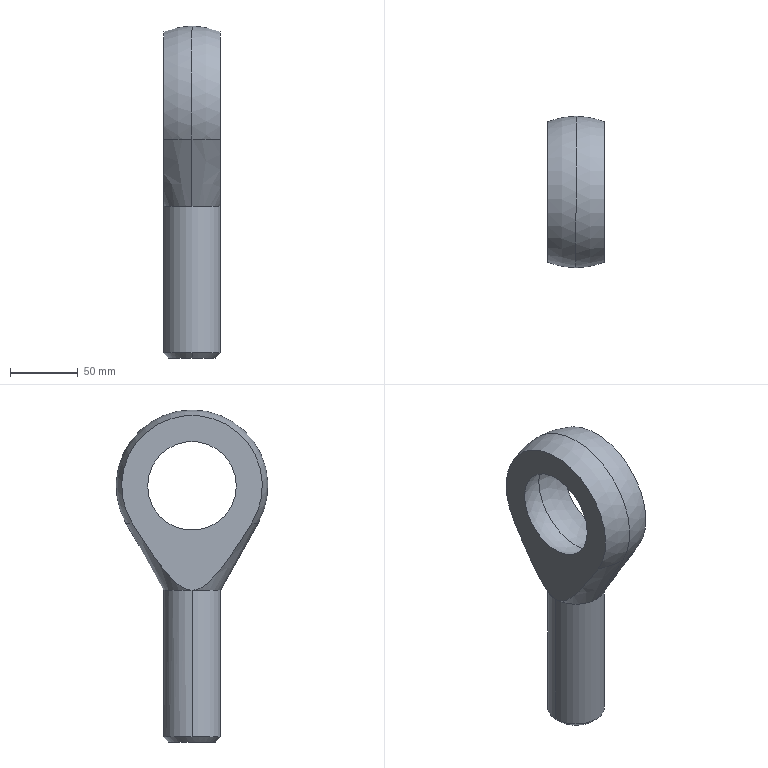Part | STEP file | Traction rod end | 1 solid | 14 faces | box 42 x 112 x 245 mm | volume 426798 mm3 | cone 5 | sphere 4 | plane 3 | cylinder 2 | commonest cylinder face diameters 42 x2
STEP:
#1=CARTESIAN_POINT('',(0.,-21.,224.245));
#2=VERTEX_POINT('',#1);
#3=CARTESIAN_POINT('',(-21.,0.,224.245));
#4=VERTEX_POINT('',#3);
#5=CARTESIAN_POINT('',(0.,0.,224.245));
#6=DIRECTION('',(0.,0.,-1.));
#7=DIRECTION('',(1.,0.,0.));
#8=AXIS2_PLACEMENT_3D('',#5,#6,#7);
#9=CIRCLE('',#8,21.);
#10=EDGE_CURVE('',#2,#4,#9,.T.);
#11=ORIENTED_EDGE('',*,*,#10,.T.);
#12=CARTESIAN_POINT('',(-21.,0.,116.002));
#13=VERTEX_POINT('',#12);
#14=CARTESIAN_POINT('',(-21.,0.,112.245));
#15=DIRECTION('',(0.,0.,-1.));
#16=VECTOR('',#15,1000.);
#17=LINE('',#14,#16);
#18=EDGE_CURVE('',#4,#13,#17,.T.);
#19=ORIENTED_EDGE('',*,*,#18,.T.);
#20=CARTESIAN_POINT('',(0.,-21.,116.002));
#21=VERTEX_POINT('',#20);
#22=CARTESIAN_POINT('',(0.,0.,116.002));
#23=DIRECTION('',(0.,0.,1.));
#24=DIRECTION('',(1.,0.,0.));
#25=AXIS2_PLACEMENT_3D('',#22,#23,#24);
#26=CIRCLE('',#25,21.);
#27=EDGE_CURVE('',#13,#21,#26,.T.);
#28=ORIENTED_EDGE('',*,*,#27,.T.);
#29=CARTESIAN_POINT('',(21.,0.,116.002));
#30=VERTEX_POINT('',#29);
#31=CARTESIAN_POINT('',(0.,0.,116.002));
#32=DIRECTION('',(0.,0.,1.));
#33=DIRECTION('',(1.,0.,0.));
#34=AXIS2_PLACEMENT_3D('',#31,#32,#33);
#35=CIRCLE('',#34,21.);
#36=EDGE_CURVE('',#21,#30,#35,.T.);
#37=ORIENTED_EDGE('',*,*,#36,.T.);
#38=CARTESIAN_POINT('',(21.,0.,224.245));
#39=VERTEX_POINT('',#38);
#40=CARTESIAN_POINT('',(21.,0.,112.245));
#41=DIRECTION('',(0.,0.,-1.));
#42=VECTOR('',#41,1000.);
#43=LINE('',#40,#42);
#44=EDGE_CURVE('',#39,#30,#43,.T.);
#45=ORIENTED_EDGE('',*,*,#44,.F.);
#46=CARTESIAN_POINT('',(0.,0.,224.245));
#47=DIRECTION('',(0.,0.,-1.));
#48=DIRECTION('',(1.,0.,0.));
#49=AXIS2_PLACEMENT_3D('',#46,#47,#48);
#50=CIRCLE('',#49,21.);
#51=EDGE_CURVE('',#39,#2,#50,.T.);
#52=ORIENTED_EDGE('',*,*,#51,.T.);
#53=EDGE_LOOP('',(#11,#19,#28,#37,#45,#52));
#54=FACE_OUTER_BOUND('',#53,.T.);
#55=CARTESIAN_POINT('',(0.,0.,112.245));
#56=DIRECTION('',(0.,0.,-1.));
#57=DIRECTION('',(1.,0.,0.));
#58=AXIS2_PLACEMENT_3D('',#55,#56,#57);
#59=CYLINDRICAL_SURFACE('',#58,21.);
#60=ADVANCED_FACE('',(#54),#59,.T.);
#61=CARTESIAN_POINT('',(0.,-17.243,112.245));
#62=VERTEX_POINT('',#61);
#63=CARTESIAN_POINT('',(0.,17.243,112.245));
#64=VERTEX_POINT('',#63);
#65=CARTESIAN_POINT('',(0.,0.,112.245));
#66=DIRECTION('',(0.,0.,1.));
#67=DIRECTION('',(0.,-1.,0.));
#68=AXIS2_PLACEMENT_3D('',#65,#66,#67);
#69=CIRCLE('',#68,17.243);
#70=EDGE_CURVE('',#62,#64,#69,.T.);
#71=ORIENTED_EDGE('',*,*,#70,.T.);
#72=CARTESIAN_POINT('',(0.,21.,116.002));
#73=VERTEX_POINT('',#72);
#74=CARTESIAN_POINT('',(0.,21.,116.002));
#75=DIRECTION('',(0.,0.7071,0.7071));
#76=VECTOR('',#75,1000.);
#77=LINE('',#74,#76);
#78=EDGE_CURVE('',#64,#73,#77,.T.);
#79=ORIENTED_EDGE('',*,*,#78,.T.);
#80=CARTESIAN_POINT('',(0.,0.,116.002));
#81=DIRECTION('',(0.,0.,1.));
#82=DIRECTION('',(1.,0.,0.));
#83=AXIS2_PLACEMENT_3D('',#80,#81,#82);
#84=CIRCLE('',#83,21.);
#85=EDGE_CURVE('',#30,#73,#84,.T.);
#86=ORIENTED_EDGE('',*,*,#85,.F.);
#87=ORIENTED_EDGE('',*,*,#36,.F.);
#88=CARTESIAN_POINT('',(0.,-21.,116.002));
#89=DIRECTION('',(0.,-0.7071,0.7071));
#90=VECTOR('',#89,1000.);
#91=LINE('',#88,#90);
#92=EDGE_CURVE('',#62,#21,#91,.T.);
#93=ORIENTED_EDGE('',*,*,#92,.F.);
#94=EDGE_LOOP('',(#71,#79,#86,#87,#93));
#95=FACE_OUTER_BOUND('',#94,.T.);
#96=CARTESIAN_POINT('',(0.,0.,116.002));
#97=DIRECTION('',(0.,0.,1.));
#98=DIRECTION('',(0.,-1.,0.));
#99=AXIS2_PLACEMENT_3D('',#96,#97,#98);
#100=CONICAL_SURFACE('',#99,21.,0.7854);
#101=ADVANCED_FACE('',(#95),#100,.T.);
#102=ORIENTED_EDGE('',*,*,#10,.F.);
#103=CARTESIAN_POINT('',(0.,-48.834,273.836));
#104=VERTEX_POINT('',#103);
#105=CARTESIAN_POINT('',(0.,-48.834,273.836));
#106=DIRECTION('',(0.,-0.4894,0.872));
#107=VECTOR('',#106,1000.);
#108=LINE('',#105,#107);
#109=EDGE_CURVE('',#2,#104,#108,.T.);
#110=ORIENTED_EDGE('',*,*,#109,.T.);
#111=CARTESIAN_POINT('',(-21.,-44.088,273.836));
#112=VERTEX_POINT('',#111);
#113=CARTESIAN_POINT('',(0.,0.,273.836));
#114=DIRECTION('',(0.,0.,-1.));
#115=DIRECTION('',(1.,0.,0.));
#116=AXIS2_PLACEMENT_3D('',#113,#114,#115);
#117=CIRCLE('',#116,48.834);
#118=EDGE_CURVE('',#104,#112,#117,.T.);
#119=ORIENTED_EDGE('',*,*,#118,.T.);
#120=CARTESIAN_POINT('',(-21.,-44.088,273.836));
#121=CARTESIAN_POINT('',(-21.,-41.092,269.018));
#122=CARTESIAN_POINT('',(-21.,-38.059,264.224));
#123=CARTESIAN_POINT('',(-21.,-33.398,257.105));
#124=CARTESIAN_POINT('',(-21.,-31.825,254.744));
#125=CARTESIAN_POINT('',(-21.,-28.623,250.059));
#126=CARTESIAN_POINT('',(-21.,-26.995,247.737));
#127=CARTESIAN_POINT('',(-21.,-23.654,243.154));
#128=CARTESIAN_POINT('',(-21.,-21.94,240.891));
#129=CARTESIAN_POINT('',(-21.,-19.26,237.586));
#130=CARTESIAN_POINT('',(-21.,-18.35,236.5));
#131=CARTESIAN_POINT('',(-21.,-16.482,234.375));
#132=CARTESIAN_POINT('',(-21.,-15.524,233.335));
#133=CARTESIAN_POINT('',(-21.,-13.538,231.323));
#134=CARTESIAN_POINT('',(-21.,-12.511,230.349));
#135=CARTESIAN_POINT('',(-21.,-10.889,228.967));
#136=CARTESIAN_POINT('',(-21.,-10.333,228.519));
#137=CARTESIAN_POINT('',(-21.,-9.193,227.663));
#138=CARTESIAN_POINT('',(-21.,-8.61,227.255));
#139=CARTESIAN_POINT('',(-21.,-7.411,226.494));
#140=CARTESIAN_POINT('',(-21.,-6.796,226.14));
#141=CARTESIAN_POINT('',(-21.,-5.522,225.502));
#142=CARTESIAN_POINT('',(-21.,-4.861,225.217));
#143=CARTESIAN_POINT('',(-21.,-3.519,224.749));
#144=CARTESIAN_POINT('',(-21.,-2.836,224.564));
#145=CARTESIAN_POINT('',(-21.,-1.438,224.312));
#146=CARTESIAN_POINT('',(-21.,-0.719,224.245));
#147=CARTESIAN_POINT('',(-21.,0.,224.245));
#148=B_SPLINE_CURVE_WITH_KNOTS('',3,(#120,#121,#122,#123,#124,#125,#126,#127,#128,#129,#130,#131,#132,#133,#134,#135,#136,#137,#138,#139,#140,#141,#142,#143,#144,#145,#146,#147),.UNSPECIFIED.,.F.,.F.,(4,2,2,2,2,2,2,2,2,2,2,2,2,4),(0.,0.01702,0.02553,0.03404,0.04255,0.0468,0.05105,0.05531,0.05744,0.05956,0.06169,0.06382,0.06595,0.06807),.UNSPECIFIED.);
#149=EDGE_CURVE('',#112,#4,#148,.T.);
#150=ORIENTED_EDGE('',*,*,#149,.T.);
#151=EDGE_LOOP('',(#102,#110,#119,#150));
#152=FACE_OUTER_BOUND('',#151,.T.);
#153=CARTESIAN_POINT('',(0.,0.,273.836));
#154=DIRECTION('',(0.,0.,1.));
#155=DIRECTION('',(0.,-1.,0.));
#156=AXIS2_PLACEMENT_3D('',#153,#154,#155);
#157=CONICAL_SURFACE('',#156,48.834,0.5115);
#158=ADVANCED_FACE('',(#152),#157,.T.);
#159=CARTESIAN_POINT('',(0.,48.834,273.836));
#160=VERTEX_POINT('',#159);
#161=CARTESIAN_POINT('',(21.,44.088,273.836));
#162=VERTEX_POINT('',#161);
#163=CARTESIAN_POINT('',(0.,0.,273.836));
#164=DIRECTION('',(0.,0.,-1.));
#165=DIRECTION('',(0.,-1.,0.));
#166=AXIS2_PLACEMENT_3D('',#163,#164,#165);
#167=CIRCLE('',#166,48.834);
#168=EDGE_CURVE('',#160,#162,#167,.T.);
#169=ORIENTED_EDGE('',*,*,#168,.F.);
#170=CARTESIAN_POINT('',(0.,0.,357.245));
#171=VERTEX_POINT('',#170);
#172=CARTESIAN_POINT('',(0.,0.,301.245));
#173=DIRECTION('',(1.,0.,0.));
#174=DIRECTION('',(0.,1.,0.));
#175=AXIS2_PLACEMENT_3D('',#172,#173,#174);
#176=CIRCLE('',#175,56.);
#177=EDGE_CURVE('',#160,#171,#176,.T.);
#178=ORIENTED_EDGE('',*,*,#177,.T.);
#179=CARTESIAN_POINT('',(0.,0.,301.245));
#180=DIRECTION('',(-1.,0.,0.));
#181=DIRECTION('',(0.,-1.,0.));
#182=AXIS2_PLACEMENT_3D('',#179,#180,#181);
#183=CIRCLE('',#182,56.);
#184=EDGE_CURVE('',#104,#171,#183,.T.);
#185=ORIENTED_EDGE('',*,*,#184,.F.);
#186=CARTESIAN_POINT('',(21.,-44.088,273.836));
#187=VERTEX_POINT('',#186);
#188=CARTESIAN_POINT('',(0.,0.,273.836));
#189=DIRECTION('',(0.,0.,-1.));
#190=DIRECTION('',(1.,0.,0.));
#191=AXIS2_PLACEMENT_3D('',#188,#189,#190);
#192=CIRCLE('',#191,48.834);
#193=EDGE_CURVE('',#187,#104,#192,.T.);
#194=ORIENTED_EDGE('',*,*,#193,.F.);
#195=CARTESIAN_POINT('',(21.,0.,301.245));
#196=DIRECTION('',(-1.,0.,0.));
#197=DIRECTION('',(0.,-1.,0.));
#198=AXIS2_PLACEMENT_3D('',#195,#196,#197);
#199=CIRCLE('',#198,51.913);
#200=EDGE_CURVE('',#187,#162,#199,.T.);
#201=ORIENTED_EDGE('',*,*,#200,.T.);
#202=EDGE_LOOP('',(#169,#178,#185,#194,#201));
#203=FACE_OUTER_BOUND('',#202,.T.);
#204=CARTESIAN_POINT('',(0.,0.,301.245));
#205=DIRECTION('',(1.,0.,0.));
#206=DIRECTION('',(0.,-1.,0.));
#207=AXIS2_PLACEMENT_3D('',#204,#205,#206);
#208=SPHERICAL_SURFACE('',#207,56.);
#209=ADVANCED_FACE('',(#203),#208,.T.);
#210=CARTESIAN_POINT('',(21.,-32.748,301.245));
#211=VERTEX_POINT('',#210);
#212=CARTESIAN_POINT('',(21.,32.748,301.245));
#213=VERTEX_POINT('',#212);
#214=CARTESIAN_POINT('',(21.,0.,301.245));
#215=DIRECTION('',(-1.,0.,0.));
#216=DIRECTION('',(0.,-1.,0.));
#217=AXIS2_PLACEMENT_3D('',#214,#215,#216);
#218=CIRCLE('',#217,32.748);
#219=EDGE_CURVE('',#211,#213,#218,.T.);
#220=ORIENTED_EDGE('',*,*,#219,.F.);
#221=CARTESIAN_POINT('',(21.,0.,301.245));
#222=DIRECTION('',(-1.,0.,0.));
#223=DIRECTION('',(0.,-1.,0.));
#224=AXIS2_PLACEMENT_3D('',#221,#222,#223);
#225=CIRCLE('',#224,32.748);
#226=EDGE_CURVE('',#213,#211,#225,.T.);
#227=ORIENTED_EDGE('',*,*,#226,.F.);
#228=EDGE_LOOP('',(#220,#227));
#229=FACE_BOUND('',#228,.T.);
#230=CARTESIAN_POINT('',(0.,0.,262.343));
#231=VERTEX_POINT('',#230);
#232=CARTESIAN_POINT('',(0.,0.,340.148));
#233=VERTEX_POINT('',#232);
#234=CARTESIAN_POINT('',(0.,0.,301.245));
#235=DIRECTION('',(1.,0.,0.));
#236=DIRECTION('',(0.,1.,0.));
#237=AXIS2_PLACEMENT_3D('',#234,#235,#236);
#238=CIRCLE('',#237,38.902);
#239=EDGE_CURVE('',#231,#233,#238,.T.);
#240=ORIENTED_EDGE('',*,*,#239,.F.);
#241=CARTESIAN_POINT('',(0.,0.,301.245));
#242=DIRECTION('',(-1.,0.,0.));
#243=DIRECTION('',(0.,-1.,0.));
#244=AXIS2_PLACEMENT_3D('',#241,#242,#243);
#245=CIRCLE('',#244,38.902);
#246=EDGE_CURVE('',#231,#233,#245,.T.);
#247=ORIENTED_EDGE('',*,*,#246,.T.);
#248=EDGE_LOOP('',(#240,#247));
#249=FACE_OUTER_BOUND('',#248,.T.);
#250=CARTESIAN_POINT('',(0.,0.,301.245));
#251=DIRECTION('',(-1.,0.,0.));
#252=DIRECTION('',(0.,1.,0.));
#253=AXIS2_PLACEMENT_3D('',#250,#251,#252);
#254=SPHERICAL_SURFACE('',#253,38.902);
#255=ADVANCED_FACE('',(#229,#249),#254,.F.);
#256=ORIENTED_EDGE('',*,*,#18,.F.);
#257=CARTESIAN_POINT('',(0.,0.,224.245));
#258=DIRECTION('',(0.,0.,-1.));
#259=DIRECTION('',(1.,0.,0.));
#260=AXIS2_PLACEMENT_3D('',#257,#258,#259);
#261=CIRCLE('',#260,21.);
#262=EDGE_CURVE('',#4,#39,#261,.T.);
#263=ORIENTED_EDGE('',*,*,#262,.T.);
#264=ORIENTED_EDGE('',*,*,#44,.T.);
#265=ORIENTED_EDGE('',*,*,#85,.T.);
#266=CARTESIAN_POINT('',(0.,0.,116.002));
#267=DIRECTION('',(0.,0.,1.));
#268=DIRECTION('',(1.,0.,0.));
#269=AXIS2_PLACEMENT_3D('',#266,#267,#268);
#270=CIRCLE('',#269,21.);
#271=EDGE_CURVE('',#73,#13,#270,.T.);
#272=ORIENTED_EDGE('',*,*,#271,.T.);
#273=EDGE_LOOP('',(#256,#263,#264,#265,#272));
#274=FACE_OUTER_BOUND('',#273,.T.);
#275=CARTESIAN_POINT('',(0.,0.,112.245));
#276=DIRECTION('',(0.,0.,-1.));
#277=DIRECTION('',(1.,0.,0.));
#278=AXIS2_PLACEMENT_3D('',#275,#276,#277);
#279=CYLINDRICAL_SURFACE('',#278,21.);
#280=ADVANCED_FACE('',(#274),#279,.T.);
#281=ORIENTED_EDGE('',*,*,#78,.F.);
#282=CARTESIAN_POINT('',(0.,0.,112.245));
#283=DIRECTION('',(0.,0.,1.));
#284=DIRECTION('',(0.,-1.,0.));
#285=AXIS2_PLACEMENT_3D('',#282,#283,#284);
#286=CIRCLE('',#285,17.243);
#287=EDGE_CURVE('',#64,#62,#286,.T.);
#288=ORIENTED_EDGE('',*,*,#287,.T.);
#289=ORIENTED_EDGE('',*,*,#92,.T.);
#290=ORIENTED_EDGE('',*,*,#27,.F.);
#291=ORIENTED_EDGE('',*,*,#271,.F.);
#292=EDGE_LOOP('',(#281,#288,#289,#290,#291));
#293=FACE_OUTER_BOUND('',#292,.T.);
#294=CARTESIAN_POINT('',(0.,0.,116.002));
#295=DIRECTION('',(0.,0.,1.));
#296=DIRECTION('',(0.,-1.,0.));
#297=AXIS2_PLACEMENT_3D('',#294,#295,#296);
#298=CONICAL_SURFACE('',#297,21.,0.7854);
#299=ADVANCED_FACE('',(#293),#298,.T.);
#300=ORIENTED_EDGE('',*,*,#109,.F.);
#301=ORIENTED_EDGE('',*,*,#51,.F.);
#302=CARTESIAN_POINT('',(21.,0.,224.245));
#303=CARTESIAN_POINT('',(21.,-1.452,224.245));
#304=CARTESIAN_POINT('',(21.,-2.851,224.514));
#305=CARTESIAN_POINT('',(21.,-4.549,225.108));
#306=CARTESIAN_POINT('',(21.,-4.887,225.241));
#307=CARTESIAN_POINT('',(21.,-5.549,225.525));
#308=CARTESIAN_POINT('',(21.,-5.873,225.677));
#309=CARTESIAN_POINT('',(21.,-6.831,226.16));
#310=CARTESIAN_POINT('',(21.,-7.449,226.517));
#311=CARTESIAN_POINT('',(21.,-8.652,227.284));
#312=CARTESIAN_POINT('',(21.,-9.237,227.694));
#313=CARTESIAN_POINT('',(21.,-10.382,228.557));
#314=CARTESIAN_POINT('',(21.,-10.942,229.011));
#315=CARTESIAN_POINT('',(21.,-12.573,230.405));
#316=CARTESIAN_POINT('',(21.,-13.601,231.384));
#317=CARTESIAN_POINT('',(21.,-15.586,233.402));
#318=CARTESIAN_POINT('',(21.,-16.542,234.442));
#319=CARTESIAN_POINT('',(21.,-18.404,236.564));
#320=CARTESIAN_POINT('',(21.,-19.31,237.646));
#321=CARTESIAN_POINT('',(21.,-21.974,240.936));
#322=CARTESIAN_POINT('',(21.,-23.681,243.189));
#323=CARTESIAN_POINT('',(21.,-27.013,247.762));
#324=CARTESIAN_POINT('',(21.,-28.64,250.084));
#325=CARTESIAN_POINT('',(21.,-31.838,254.764));
#326=CARTESIAN_POINT('',(21.,-33.409,257.122));
#327=CARTESIAN_POINT('',(21.,-38.065,264.234));
#328=CARTESIAN_POINT('',(21.,-41.095,269.023));
#329=CARTESIAN_POINT('',(21.,-44.088,273.836));
#330=B_SPLINE_CURVE_WITH_KNOTS('',3,(#302,#303,#304,#305,#306,#307,#308,#309,#310,#311,#312,#313,#314,#315,#316,#317,#318,#319,#320,#321,#322,#323,#324,#325,#326,#327,#328,#329),.UNSPECIFIED.,.F.,.F.,(4,2,2,2,2,2,2,2,2,2,2,2,2,4),(0.,0.004274,0.005342,0.006411,0.008548,0.01068,0.01282,0.0171,0.02137,0.02564,0.03419,0.04274,0.05129,0.06838),.UNSPECIFIED.);
#331=EDGE_CURVE('',#39,#187,#330,.T.);
#332=ORIENTED_EDGE('',*,*,#331,.T.);
#333=ORIENTED_EDGE('',*,*,#193,.T.);
#334=EDGE_LOOP('',(#300,#301,#332,#333));
#335=FACE_OUTER_BOUND('',#334,.T.);
#336=CARTESIAN_POINT('',(0.,0.,273.836));
#337=DIRECTION('',(0.,0.,1.));
#338=DIRECTION('',(0.,-1.,0.));
#339=AXIS2_PLACEMENT_3D('',#336,#337,#338);
#340=CONICAL_SURFACE('',#339,48.834,0.5115);
#341=ADVANCED_FACE('',(#335),#340,.T.);
#342=ORIENTED_EDGE('',*,*,#70,.F.);
#343=ORIENTED_EDGE('',*,*,#287,.F.);
#344=EDGE_LOOP('',(#342,#343));
#345=FACE_OUTER_BOUND('',#344,.T.);
#346=CARTESIAN_POINT('',(-17.243,0.,112.245));
#347=DIRECTION('',(0.,0.,1.));
#348=DIRECTION('',(-1.,0.,0.));
#349=AXIS2_PLACEMENT_3D('',#346,#347,#348);
#350=PLANE('',#349);
#351=ADVANCED_FACE('',(#345),#350,.F.);
#352=CARTESIAN_POINT('',(21.,44.088,273.836));
#353=CARTESIAN_POINT('',(21.,41.092,269.018));
#354=CARTESIAN_POINT('',(21.,38.059,264.224));
#355=CARTESIAN_POINT('',(21.,33.398,257.105));
#356=CARTESIAN_POINT('',(21.,31.825,254.744));
#357=CARTESIAN_POINT('',(21.,28.623,250.059));
#358=CARTESIAN_POINT('',(21.,26.995,247.737));
#359=CARTESIAN_POINT('',(21.,23.654,243.154));
#360=CARTESIAN_POINT('',(21.,21.94,240.891));
#361=CARTESIAN_POINT('',(21.,19.26,237.586));
#362=CARTESIAN_POINT('',(21.,18.35,236.5));
#363=CARTESIAN_POINT('',(21.,16.482,234.375));
#364=CARTESIAN_POINT('',(21.,15.524,233.335));
#365=CARTESIAN_POINT('',(21.,13.538,231.323));
#366=CARTESIAN_POINT('',(21.,12.511,230.349));
#367=CARTESIAN_POINT('',(21.,10.889,228.967));
#368=CARTESIAN_POINT('',(21.,10.333,228.519));
#369=CARTESIAN_POINT('',(21.,9.193,227.663));
#370=CARTESIAN_POINT('',(21.,8.61,227.255));
#371=CARTESIAN_POINT('',(21.,7.411,226.494));
#372=CARTESIAN_POINT('',(21.,6.796,226.14));
#373=CARTESIAN_POINT('',(21.,5.522,225.502));
#374=CARTESIAN_POINT('',(21.,4.861,225.217));
#375=CARTESIAN_POINT('',(21.,3.519,224.749));
#376=CARTESIAN_POINT('',(21.,2.836,224.564));
#377=CARTESIAN_POINT('',(21.,1.438,224.312));
#378=CARTESIAN_POINT('',(21.,0.719,224.245));
#379=CARTESIAN_POINT('',(21.,0.,224.245));
#380=B_SPLINE_CURVE_WITH_KNOTS('',3,(#352,#353,#354,#355,#356,#357,#358,#359,#360,#361,#362,#363,#364,#365,#366,#367,#368,#369,#370,#371,#372,#373,#374,#375,#376,#377,#378,#379),.UNSPECIFIED.,.F.,.F.,(4,2,2,2,2,2,2,2,2,2,2,2,2,4),(0.,0.01702,0.02553,0.03404,0.04255,0.0468,0.05105,0.05531,0.05744,0.05956,0.06169,0.06382,0.06595,0.06807),.UNSPECIFIED.);
#381=EDGE_CURVE('',#162,#39,#380,.T.);
#382=ORIENTED_EDGE('',*,*,#381,.T.);
#383=ORIENTED_EDGE('',*,*,#262,.F.);
#384=CARTESIAN_POINT('',(-21.,44.088,273.836));
#385=VERTEX_POINT('',#384);
#386=CARTESIAN_POINT('',(-21.,0.,224.245));
#387=CARTESIAN_POINT('',(-21.,1.452,224.245));
#388=CARTESIAN_POINT('',(-21.,2.851,224.514));
#389=CARTESIAN_POINT('',(-21.,4.549,225.108));
#390=CARTESIAN_POINT('',(-21.,4.887,225.241));
#391=CARTESIAN_POINT('',(-21.,5.549,225.525));
#392=CARTESIAN_POINT('',(-21.,5.873,225.677));
#393=CARTESIAN_POINT('',(-21.,6.831,226.16));
#394=CARTESIAN_POINT('',(-21.,7.449,226.517));
#395=CARTESIAN_POINT('',(-21.,8.652,227.284));
#396=CARTESIAN_POINT('',(-21.,9.237,227.694));
#397=CARTESIAN_POINT('',(-21.,10.382,228.557));
#398=CARTESIAN_POINT('',(-21.,10.942,229.011));
#399=CARTESIAN_POINT('',(-21.,12.573,230.405));
#400=CARTESIAN_POINT('',(-21.,13.601,231.384));
#401=CARTESIAN_POINT('',(-21.,15.586,233.402));
#402=CARTESIAN_POINT('',(-21.,16.542,234.442));
#403=CARTESIAN_POINT('',(-21.,18.404,236.564));
#404=CARTESIAN_POINT('',(-21.,19.31,237.646));
#405=CARTESIAN_POINT('',(-21.,21.974,240.936));
#406=CARTESIAN_POINT('',(-21.,23.681,243.189));
#407=CARTESIAN_POINT('',(-21.,27.013,247.762));
#408=CARTESIAN_POINT('',(-21.,28.64,250.084));
#409=CARTESIAN_POINT('',(-21.,31.838,254.764));
#410=CARTESIAN_POINT('',(-21.,33.409,257.122));
#411=CARTESIAN_POINT('',(-21.,38.065,264.234));
#412=CARTESIAN_POINT('',(-21.,41.095,269.023));
#413=CARTESIAN_POINT('',(-21.,44.088,273.836));
#414=B_SPLINE_CURVE_WITH_KNOTS('',3,(#386,#387,#388,#389,#390,#391,#392,#393,#394,#395,#396,#397,#398,#399,#400,#401,#402,#403,#404,#405,#406,#407,#408,#409,#410,#411,#412,#413),.UNSPECIFIED.,.F.,.F.,(4,2,2,2,2,2,2,2,2,2,2,2,2,4),(0.,0.004274,0.005342,0.006411,0.008548,0.01068,0.01282,0.0171,0.02137,0.02564,0.03419,0.04274,0.05129,0.06838),.UNSPECIFIED.);
#415=EDGE_CURVE('',#4,#385,#414,.T.);
#416=ORIENTED_EDGE('',*,*,#415,.T.);
#417=CARTESIAN_POINT('',(0.,0.,273.836));
#418=DIRECTION('',(0.,0.,-1.));
#419=DIRECTION('',(0.,-1.,0.));
#420=AXIS2_PLACEMENT_3D('',#417,#418,#419);
#421=CIRCLE('',#420,48.834);
#422=EDGE_CURVE('',#385,#160,#421,.T.);
#423=ORIENTED_EDGE('',*,*,#422,.T.);
#424=ORIENTED_EDGE('',*,*,#168,.T.);
#425=EDGE_LOOP('',(#382,#383,#416,#423,#424));
#426=FACE_OUTER_BOUND('',#425,.T.);
#427=CARTESIAN_POINT('',(0.,0.,273.836));
#428=DIRECTION('',(0.,0.,1.));
#429=DIRECTION('',(0.,-1.,0.));
#430=AXIS2_PLACEMENT_3D('',#427,#428,#429);
#431=CONICAL_SURFACE('',#430,48.834,0.5115);
#432=ADVANCED_FACE('',(#426),#431,.T.);
#433=ORIENTED_EDGE('',*,*,#177,.F.);
#434=ORIENTED_EDGE('',*,*,#422,.F.);
#435=CARTESIAN_POINT('',(-21.,0.,301.245));
#436=DIRECTION('',(1.,0.,0.));
#437=DIRECTION('',(0.,1.,0.));
#438=AXIS2_PLACEMENT_3D('',#435,#436,#437);
#439=CIRCLE('',#438,51.913);
#440=EDGE_CURVE('',#385,#112,#439,.T.);
#441=ORIENTED_EDGE('',*,*,#440,.T.);
#442=ORIENTED_EDGE('',*,*,#118,.F.);
#443=ORIENTED_EDGE('',*,*,#184,.T.);
#444=EDGE_LOOP('',(#433,#434,#441,#442,#443));
#445=FACE_OUTER_BOUND('',#444,.T.);
#446=CARTESIAN_POINT('',(0.,0.,301.245));
#447=DIRECTION('',(1.,0.,0.));
#448=DIRECTION('',(0.,-1.,0.));
#449=AXIS2_PLACEMENT_3D('',#446,#447,#448);
#450=SPHERICAL_SURFACE('',#449,56.);
#451=ADVANCED_FACE('',(#445),#450,.T.);
#452=ORIENTED_EDGE('',*,*,#219,.T.);
#453=ORIENTED_EDGE('',*,*,#226,.T.);
#454=EDGE_LOOP('',(#452,#453));
#455=FACE_BOUND('',#454,.T.);
#456=ORIENTED_EDGE('',*,*,#381,.F.);
#457=ORIENTED_EDGE('',*,*,#200,.F.);
#458=ORIENTED_EDGE('',*,*,#331,.F.);
#459=EDGE_LOOP('',(#456,#457,#458));
#460=FACE_OUTER_BOUND('',#459,.T.);
#461=CARTESIAN_POINT('',(21.,0.,353.158));
#462=DIRECTION('',(1.,0.,0.));
#463=DIRECTION('',(0.,-1.,0.));
#464=AXIS2_PLACEMENT_3D('',#461,#462,#463);
#465=PLANE('',#464);
#466=ADVANCED_FACE('',(#455,#460),#465,.T.);
#467=ORIENTED_EDGE('',*,*,#415,.F.);
#468=ORIENTED_EDGE('',*,*,#149,.F.);
#469=ORIENTED_EDGE('',*,*,#440,.F.);
#470=EDGE_LOOP('',(#467,#468,#469));
#471=FACE_OUTER_BOUND('',#470,.T.);
#472=CARTESIAN_POINT('',(-21.,32.748,301.245));
#473=VERTEX_POINT('',#472);
#474=CARTESIAN_POINT('',(-21.,-32.748,301.245));
#475=VERTEX_POINT('',#474);
#476=CARTESIAN_POINT('',(-21.,0.,301.245));
#477=DIRECTION('',(1.,0.,0.));
#478=DIRECTION('',(0.,1.,0.));
#479=AXIS2_PLACEMENT_3D('',#476,#477,#478);
#480=CIRCLE('',#479,32.748);
#481=EDGE_CURVE('',#473,#475,#480,.T.);
#482=ORIENTED_EDGE('',*,*,#481,.T.);
#483=CARTESIAN_POINT('',(-21.,0.,301.245));
#484=DIRECTION('',(1.,0.,0.));
#485=DIRECTION('',(0.,1.,0.));
#486=AXIS2_PLACEMENT_3D('',#483,#484,#485);
#487=CIRCLE('',#486,32.748);
#488=EDGE_CURVE('',#475,#473,#487,.T.);
#489=ORIENTED_EDGE('',*,*,#488,.T.);
#490=EDGE_LOOP('',(#482,#489));
#491=FACE_BOUND('',#490,.T.);
#492=CARTESIAN_POINT('',(-21.,0.,333.993));
#493=DIRECTION('',(-1.,0.,0.));
#494=DIRECTION('',(0.,1.,0.));
#495=AXIS2_PLACEMENT_3D('',#492,#493,#494);
#496=PLANE('',#495);
#497=ADVANCED_FACE('',(#471,#491),#496,.T.);
#498=ORIENTED_EDGE('',*,*,#246,.F.);
#499=ORIENTED_EDGE('',*,*,#239,.T.);
#500=EDGE_LOOP('',(#498,#499));
#501=FACE_OUTER_BOUND('',#500,.T.);
#502=ORIENTED_EDGE('',*,*,#481,.F.);
#503=ORIENTED_EDGE('',*,*,#488,.F.);
#504=EDGE_LOOP('',(#502,#503));
#505=FACE_BOUND('',#504,.T.);
#506=CARTESIAN_POINT('',(0.,0.,301.245));
#507=DIRECTION('',(-1.,0.,0.));
#508=DIRECTION('',(0.,1.,0.));
#509=AXIS2_PLACEMENT_3D('',#506,#507,#508);
#510=SPHERICAL_SURFACE('',#509,38.902);
#511=ADVANCED_FACE('',(#501,#505),#510,.F.);
#512=CLOSED_SHELL('',(#60,#101,#158,#209,#255,#280,#299,#341,#351,#432,#451,#466,#497,#511));
#513=MANIFOLD_SOLID_BREP('',#512);
#514=CARTESIAN_POINT('',(0.,0.,0.));
#515=DIRECTION('',(0.,0.,1.));
#516=DIRECTION('',(1.,0.,0.));
#517=AXIS2_PLACEMENT_3D('',#514,#515,#516);
#518=(LENGTH_UNIT()NAMED_UNIT(*)SI_UNIT(.MILLI.,.METRE.));
#519=UNCERTAINTY_MEASURE_WITH_UNIT(LENGTH_MEASURE(0.00001),#518,'','');
#520=(NAMED_UNIT(*)PLANE_ANGLE_UNIT()SI_UNIT($,.RADIAN.));
#521=(NAMED_UNIT(*)SI_UNIT($,.STERADIAN.)SOLID_ANGLE_UNIT());
#522=(GEOMETRIC_REPRESENTATION_CONTEXT(3)GLOBAL_UNCERTAINTY_ASSIGNED_CONTEXT((#519))GLOBAL_UNIT_ASSIGNED_CONTEXT((#518,#520,#521))REPRESENTATION_CONTEXT('',''));
#523=ADVANCED_BREP_SHAPE_REPRESENTATION('',(#513,#517),#522);